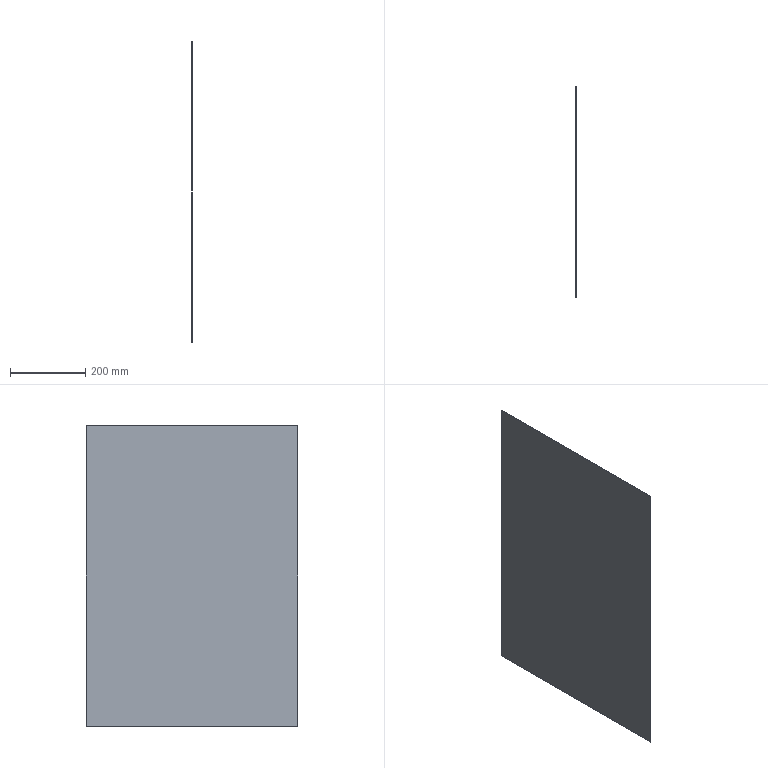Part | SolidWorks | 1 solid | 6 faces | box 1.5 x 562 x 800 mm | volume 674400 mm3 | plane 6
STEP:
#1=CARTESIAN_POINT('',(0.,281.,400.));
#2=VERTEX_POINT('',#1);
#3=CARTESIAN_POINT('',(0.,-281.,400.));
#4=VERTEX_POINT('',#3);
#5=CARTESIAN_POINT('',(0.,-281.,400.));
#6=DIRECTION('',(0.,-1.,0.));
#7=VECTOR('',#6,1000.);
#8=LINE('',#5,#7);
#9=EDGE_CURVE('',#2,#4,#8,.T.);
#10=ORIENTED_EDGE('',*,*,#9,.F.);
#11=CARTESIAN_POINT('',(-1.5,281.,400.));
#12=VERTEX_POINT('',#11);
#13=CARTESIAN_POINT('',(-1.5,281.,400.));
#14=DIRECTION('',(1.,0.,0.));
#15=VECTOR('',#14,1000.);
#16=LINE('',#13,#15);
#17=EDGE_CURVE('',#12,#2,#16,.T.);
#18=ORIENTED_EDGE('',*,*,#17,.F.);
#19=CARTESIAN_POINT('',(-1.5,-281.,400.));
#20=VERTEX_POINT('',#19);
#21=CARTESIAN_POINT('',(-1.5,-281.,400.));
#22=DIRECTION('',(0.,-1.,0.));
#23=VECTOR('',#22,1000.);
#24=LINE('',#21,#23);
#25=EDGE_CURVE('',#12,#20,#24,.T.);
#26=ORIENTED_EDGE('',*,*,#25,.T.);
#27=CARTESIAN_POINT('',(-1.5,-281.,400.));
#28=DIRECTION('',(1.,0.,0.));
#29=VECTOR('',#28,1000.);
#30=LINE('',#27,#29);
#31=EDGE_CURVE('',#20,#4,#30,.T.);
#32=ORIENTED_EDGE('',*,*,#31,.T.);
#33=EDGE_LOOP('',(#10,#18,#26,#32));
#34=FACE_OUTER_BOUND('',#33,.T.);
#35=CARTESIAN_POINT('',(-1.5,-281.,400.));
#36=DIRECTION('',(0.,0.,1.));
#37=DIRECTION('',(1.,0.,0.));
#38=AXIS2_PLACEMENT_3D('',#35,#36,#37);
#39=PLANE('',#38);
#40=ADVANCED_FACE('',(#34),#39,.T.);
#41=CARTESIAN_POINT('',(0.,281.,-400.));
#42=VERTEX_POINT('',#41);
#43=CARTESIAN_POINT('',(0.,281.,-400.));
#44=DIRECTION('',(0.,0.,1.));
#45=VECTOR('',#44,1000.);
#46=LINE('',#43,#45);
#47=EDGE_CURVE('',#42,#2,#46,.T.);
#48=ORIENTED_EDGE('',*,*,#47,.F.);
#49=CARTESIAN_POINT('',(-1.5,281.,-400.));
#50=VERTEX_POINT('',#49);
#51=CARTESIAN_POINT('',(-1.5,281.,-400.));
#52=DIRECTION('',(1.,0.,0.));
#53=VECTOR('',#52,1000.);
#54=LINE('',#51,#53);
#55=EDGE_CURVE('',#50,#42,#54,.T.);
#56=ORIENTED_EDGE('',*,*,#55,.F.);
#57=CARTESIAN_POINT('',(-1.5,281.,-400.));
#58=DIRECTION('',(0.,0.,1.));
#59=VECTOR('',#58,1000.);
#60=LINE('',#57,#59);
#61=EDGE_CURVE('',#50,#12,#60,.T.);
#62=ORIENTED_EDGE('',*,*,#61,.T.);
#63=ORIENTED_EDGE('',*,*,#17,.T.);
#64=EDGE_LOOP('',(#48,#56,#62,#63));
#65=FACE_OUTER_BOUND('',#64,.T.);
#66=CARTESIAN_POINT('',(-1.5,281.,-400.));
#67=DIRECTION('',(0.,1.,0.));
#68=DIRECTION('',(0.,0.,1.));
#69=AXIS2_PLACEMENT_3D('',#66,#67,#68);
#70=PLANE('',#69);
#71=ADVANCED_FACE('',(#65),#70,.T.);
#72=CARTESIAN_POINT('',(0.,-281.,-400.));
#73=VERTEX_POINT('',#72);
#74=CARTESIAN_POINT('',(0.,-281.,-400.));
#75=DIRECTION('',(0.,1.,0.));
#76=VECTOR('',#75,1000.);
#77=LINE('',#74,#76);
#78=EDGE_CURVE('',#73,#42,#77,.T.);
#79=ORIENTED_EDGE('',*,*,#78,.F.);
#80=CARTESIAN_POINT('',(-1.5,-281.,-400.));
#81=VERTEX_POINT('',#80);
#82=CARTESIAN_POINT('',(-1.5,-281.,-400.));
#83=DIRECTION('',(1.,0.,0.));
#84=VECTOR('',#83,1000.);
#85=LINE('',#82,#84);
#86=EDGE_CURVE('',#81,#73,#85,.T.);
#87=ORIENTED_EDGE('',*,*,#86,.F.);
#88=CARTESIAN_POINT('',(-1.5,-281.,-400.));
#89=DIRECTION('',(0.,1.,0.));
#90=VECTOR('',#89,1000.);
#91=LINE('',#88,#90);
#92=EDGE_CURVE('',#81,#50,#91,.T.);
#93=ORIENTED_EDGE('',*,*,#92,.T.);
#94=ORIENTED_EDGE('',*,*,#55,.T.);
#95=EDGE_LOOP('',(#79,#87,#93,#94));
#96=FACE_OUTER_BOUND('',#95,.T.);
#97=CARTESIAN_POINT('',(-1.5,-281.,-400.));
#98=DIRECTION('',(0.,0.,-1.));
#99=DIRECTION('',(-1.,0.,0.));
#100=AXIS2_PLACEMENT_3D('',#97,#98,#99);
#101=PLANE('',#100);
#102=ADVANCED_FACE('',(#96),#101,.T.);
#103=CARTESIAN_POINT('',(0.,-281.,-400.));
#104=DIRECTION('',(0.,0.,-1.));
#105=VECTOR('',#104,1000.);
#106=LINE('',#103,#105);
#107=EDGE_CURVE('',#4,#73,#106,.T.);
#108=ORIENTED_EDGE('',*,*,#107,.F.);
#109=ORIENTED_EDGE('',*,*,#31,.F.);
#110=CARTESIAN_POINT('',(-1.5,-281.,-400.));
#111=DIRECTION('',(0.,0.,-1.));
#112=VECTOR('',#111,1000.);
#113=LINE('',#110,#112);
#114=EDGE_CURVE('',#20,#81,#113,.T.);
#115=ORIENTED_EDGE('',*,*,#114,.T.);
#116=ORIENTED_EDGE('',*,*,#86,.T.);
#117=EDGE_LOOP('',(#108,#109,#115,#116));
#118=FACE_OUTER_BOUND('',#117,.T.);
#119=CARTESIAN_POINT('',(-1.5,-281.,-400.));
#120=DIRECTION('',(0.,-1.,0.));
#121=DIRECTION('',(0.,0.,-1.));
#122=AXIS2_PLACEMENT_3D('',#119,#120,#121);
#123=PLANE('',#122);
#124=ADVANCED_FACE('',(#118),#123,.T.);
#125=ORIENTED_EDGE('',*,*,#25,.F.);
#126=ORIENTED_EDGE('',*,*,#61,.F.);
#127=ORIENTED_EDGE('',*,*,#92,.F.);
#128=ORIENTED_EDGE('',*,*,#114,.F.);
#129=EDGE_LOOP('',(#125,#126,#127,#128));
#130=FACE_OUTER_BOUND('',#129,.T.);
#131=CARTESIAN_POINT('',(-1.5,0.,0.));
#132=DIRECTION('',(1.,0.,0.));
#133=DIRECTION('',(0.,0.,-1.));
#134=AXIS2_PLACEMENT_3D('',#131,#132,#133);
#135=PLANE('',#134);
#136=ADVANCED_FACE('',(#130),#135,.F.);
#137=ORIENTED_EDGE('',*,*,#9,.T.);
#138=ORIENTED_EDGE('',*,*,#107,.T.);
#139=ORIENTED_EDGE('',*,*,#78,.T.);
#140=ORIENTED_EDGE('',*,*,#47,.T.);
#141=EDGE_LOOP('',(#137,#138,#139,#140));
#142=FACE_OUTER_BOUND('',#141,.T.);
#143=CARTESIAN_POINT('',(0.,0.,0.));
#144=DIRECTION('',(1.,0.,0.));
#145=DIRECTION('',(0.,0.,-1.));
#146=AXIS2_PLACEMENT_3D('',#143,#144,#145);
#147=PLANE('',#146);
#148=ADVANCED_FACE('',(#142),#147,.T.);
#149=CLOSED_SHELL('',(#40,#71,#102,#124,#136,#148));
#150=MANIFOLD_SOLID_BREP('',#149);
#151=CARTESIAN_POINT('',(0.,0.,0.));
#152=DIRECTION('',(0.,0.,1.));
#153=DIRECTION('',(1.,0.,0.));
#154=AXIS2_PLACEMENT_3D('',#151,#152,#153);
#155=(LENGTH_UNIT()NAMED_UNIT(*)SI_UNIT(.MILLI.,.METRE.));
#156=UNCERTAINTY_MEASURE_WITH_UNIT(LENGTH_MEASURE(0.00001),#155,'','');
#157=(NAMED_UNIT(*)PLANE_ANGLE_UNIT()SI_UNIT($,.RADIAN.));
#158=(NAMED_UNIT(*)SI_UNIT($,.STERADIAN.)SOLID_ANGLE_UNIT());
#159=(GEOMETRIC_REPRESENTATION_CONTEXT(3)GLOBAL_UNCERTAINTY_ASSIGNED_CONTEXT((#156))GLOBAL_UNIT_ASSIGNED_CONTEXT((#155,#157,#158))REPRESENTATION_CONTEXT('',''));
#160=ADVANCED_BREP_SHAPE_REPRESENTATION('',(#150,#154),#159);